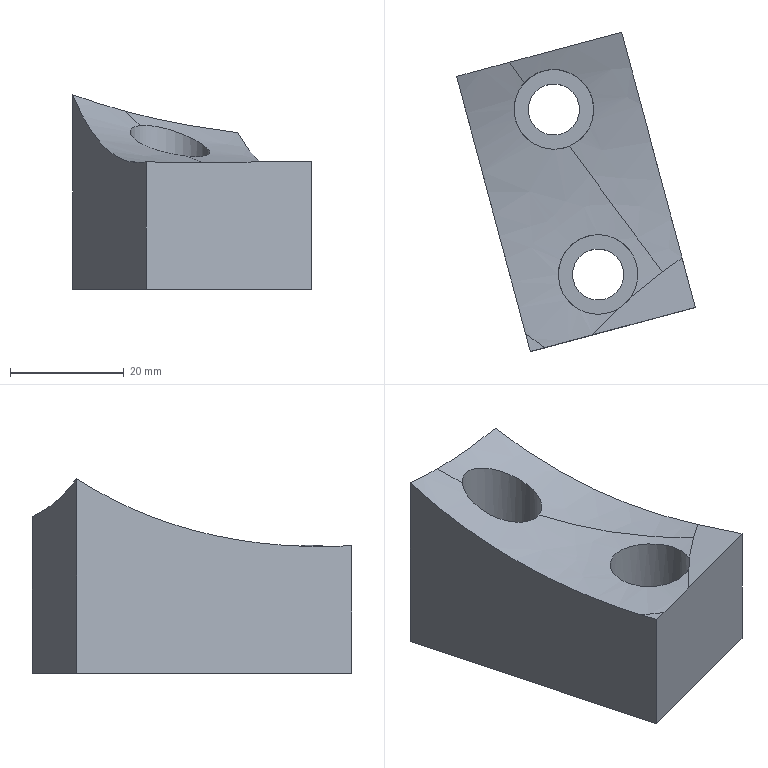Part | NX | features solid 2 | 1 solid | 15 faces | box 41.919 x 56.061 x 34.182 mm | volume 29881 mm3 | plane 7 | cylinder 4 | spline 4 | commonest cylinder face diameters 9 x2 14 x2
STEP:
#1=CARTESIAN_POINT('',(-500.421,532.504,-77.579));
#2=VERTEX_POINT('',#1);
#3=CARTESIAN_POINT('',(-497.915,533.175,-77.679));
#4=VERTEX_POINT('',#3);
#5=CARTESIAN_POINT('',(-500.421,532.504,-77.579));
#6=CARTESIAN_POINT('',(-499.586,532.727,-77.618));
#7=CARTESIAN_POINT('',(-498.751,532.951,-77.652));
#8=CARTESIAN_POINT('',(-497.915,533.175,-77.679));
#9=B_SPLINE_CURVE_WITH_KNOTS('',3,(#5,#6,#7,#8),.UNSPECIFIED.,.F.,.F.,(4,4),(0.,0.002596),.UNSPECIFIED.);
#10=EDGE_CURVE('',#2,#4,#9,.T.);
#11=ORIENTED_EDGE('',*,*,#10,.F.);
#12=CARTESIAN_POINT('',(-500.421,532.504,-100.));
#13=VERTEX_POINT('',#12);
#14=CARTESIAN_POINT('',(-500.421,532.504,-105.));
#15=DIRECTION('',(0.,0.,1.));
#16=VECTOR('',#15,1000.);
#17=LINE('',#14,#16);
#18=EDGE_CURVE('',#13,#2,#17,.T.);
#19=ORIENTED_EDGE('',*,*,#18,.F.);
#20=CARTESIAN_POINT('',(-471.443,540.268,-100.));
#21=VERTEX_POINT('',#20);
#22=CARTESIAN_POINT('',(-500.421,532.504,-100.));
#23=DIRECTION('',(0.9659,0.2588,0.));
#24=VECTOR('',#23,1000.);
#25=LINE('',#22,#24);
#26=EDGE_CURVE('',#13,#21,#25,.T.);
#27=ORIENTED_EDGE('',*,*,#26,.T.);
#28=CARTESIAN_POINT('',(-471.443,540.268,-77.491));
#29=VERTEX_POINT('',#28);
#30=CARTESIAN_POINT('',(-471.443,540.268,-105.));
#31=DIRECTION('',(0.,0.,1.));
#32=VECTOR('',#31,1000.);
#33=LINE('',#30,#32);
#34=EDGE_CURVE('',#21,#29,#33,.T.);
#35=ORIENTED_EDGE('',*,*,#34,.T.);
#36=CARTESIAN_POINT('',(-489.455,535.442,-77.745));
#37=VERTEX_POINT('',#36);
#38=CARTESIAN_POINT('',(-489.455,535.442,-77.745));
#39=CARTESIAN_POINT('',(-483.451,537.051,-77.658));
#40=CARTESIAN_POINT('',(-477.447,538.66,-77.574));
#41=CARTESIAN_POINT('',(-471.443,540.268,-77.491));
#42=B_SPLINE_CURVE_WITH_KNOTS('',3,(#38,#39,#40,#41),.UNSPECIFIED.,.F.,.F.,(4,4),(0.01135,0.03),.UNSPECIFIED.);
#43=EDGE_CURVE('',#37,#29,#42,.T.);
#44=ORIENTED_EDGE('',*,*,#43,.F.);
#45=CARTESIAN_POINT('',(-497.915,533.175,-77.679));
#46=CARTESIAN_POINT('',(-495.095,533.931,-77.77));
#47=CARTESIAN_POINT('',(-492.274,534.687,-77.786));
#48=CARTESIAN_POINT('',(-489.453,535.442,-77.745));
#49=B_SPLINE_CURVE_WITH_KNOTS('',3,(#45,#46,#47,#48),.UNSPECIFIED.,.F.,.F.,(4,4),(0.,0.008761),.UNSPECIFIED.);
#50=EDGE_CURVE('',#4,#37,#49,.T.);
#51=ORIENTED_EDGE('',*,*,#50,.F.);
#52=EDGE_LOOP('',(#11,#19,#27,#35,#44,#51));
#53=FACE_BOUND('',#52,.T.);
#54=CARTESIAN_POINT('',(-500.421,532.504,-105.));
#55=DIRECTION('',(0.2588,-0.9659,0.));
#56=DIRECTION('',(0.9659,0.2588,0.));
#57=AXIS2_PLACEMENT_3D('',#54,#55,#56);
#58=PLANE('',#57);
#59=ADVANCED_FACE('',(#53),#58,.T.);
#60=CARTESIAN_POINT('',(-473.762,548.924,-78.67));
#61=VERTEX_POINT('',#60);
#62=CARTESIAN_POINT('',(-484.384,588.565,-72.498));
#63=VERTEX_POINT('',#62);
#64=CARTESIAN_POINT('',(-473.762,548.921,-78.67));
#65=CARTESIAN_POINT('',(-475.574,555.683,-79.599));
#66=CARTESIAN_POINT('',(-478.278,565.777,-79.565));
#67=CARTESIAN_POINT('',(-481.86,579.146,-76.501));
#68=CARTESIAN_POINT('',(-483.556,585.475,-73.999));
#69=CARTESIAN_POINT('',(-484.384,588.565,-72.498));
#70=B_SPLINE_CURVE_WITH_KNOTS('',3,(#64,#65,#66,#67,#68,#69),.UNSPECIFIED.,.F.,.F.,(4,1,1,4),(0.,0.0209,0.03134,0.04179),.UNSPECIFIED.);
#71=EDGE_CURVE('',#61,#63,#70,.T.);
#72=ORIENTED_EDGE('',*,*,#71,.F.);
#73=CARTESIAN_POINT('',(-471.443,540.268,-77.491));
#74=CARTESIAN_POINT('',(-472.216,543.154,-77.881));
#75=CARTESIAN_POINT('',(-472.99,546.039,-78.274));
#76=CARTESIAN_POINT('',(-473.763,548.924,-78.67));
#77=B_SPLINE_CURVE_WITH_KNOTS('',3,(#73,#74,#75,#76),.UNSPECIFIED.,.F.,.F.,(4,4),(0.,0.009039),.UNSPECIFIED.);
#78=EDGE_CURVE('',#29,#61,#77,.T.);
#79=ORIENTED_EDGE('',*,*,#78,.F.);
#80=ORIENTED_EDGE('',*,*,#34,.F.);
#81=CARTESIAN_POINT('',(-484.384,588.565,-100.));
#82=VERTEX_POINT('',#81);
#83=CARTESIAN_POINT('',(-471.443,540.268,-100.));
#84=DIRECTION('',(-0.2588,0.9659,0.));
#85=VECTOR('',#84,1000.);
#86=LINE('',#83,#85);
#87=EDGE_CURVE('',#21,#82,#86,.T.);
#88=ORIENTED_EDGE('',*,*,#87,.T.);
#89=CARTESIAN_POINT('',(-484.384,588.565,-105.));
#90=DIRECTION('',(0.,0.,1.));
#91=VECTOR('',#90,1000.);
#92=LINE('',#89,#91);
#93=EDGE_CURVE('',#82,#63,#92,.T.);
#94=ORIENTED_EDGE('',*,*,#93,.T.);
#95=EDGE_LOOP('',(#72,#79,#80,#88,#94));
#96=FACE_BOUND('',#95,.T.);
#97=CARTESIAN_POINT('',(-471.443,540.268,-105.));
#98=DIRECTION('',(0.9659,0.2588,0.));
#99=DIRECTION('',(-0.2588,0.9659,0.));
#100=AXIS2_PLACEMENT_3D('',#97,#98,#99);
#101=PLANE('',#100);
#102=ADVANCED_FACE('',(#96),#101,.T.);
#103=CARTESIAN_POINT('',(-504.086,583.285,-68.736));
#104=VERTEX_POINT('',#103);
#105=CARTESIAN_POINT('',(-484.384,588.565,-72.498));
#106=CARTESIAN_POINT('',(-491.031,586.784,-71.689));
#107=CARTESIAN_POINT('',(-497.606,585.022,-70.481));
#108=CARTESIAN_POINT('',(-504.086,583.285,-68.736));
#109=B_SPLINE_CURVE_WITH_KNOTS('',3,(#105,#106,#107,#108),.UNSPECIFIED.,.F.,.F.,(4,4),(0.,0.02074),.UNSPECIFIED.);
#110=EDGE_CURVE('',#63,#104,#109,.T.);
#111=ORIENTED_EDGE('',*,*,#110,.F.);
#112=ORIENTED_EDGE('',*,*,#93,.F.);
#113=CARTESIAN_POINT('',(-513.362,580.8,-100.));
#114=VERTEX_POINT('',#113);
#115=CARTESIAN_POINT('',(-513.362,580.8,-100.));
#116=DIRECTION('',(-0.9659,-0.2588,0.));
#117=VECTOR('',#116,1000.);
#118=LINE('',#115,#117);
#119=EDGE_CURVE('',#114,#82,#118,.F.);
#120=ORIENTED_EDGE('',*,*,#119,.F.);
#121=CARTESIAN_POINT('',(-513.362,580.8,-65.818));
#122=VERTEX_POINT('',#121);
#123=CARTESIAN_POINT('',(-513.362,580.8,-105.));
#124=DIRECTION('',(0.,0.,1.));
#125=VECTOR('',#124,1000.);
#126=LINE('',#123,#125);
#127=EDGE_CURVE('',#114,#122,#126,.T.);
#128=ORIENTED_EDGE('',*,*,#127,.T.);
#129=CARTESIAN_POINT('',(-504.086,583.285,-68.736));
#130=CARTESIAN_POINT('',(-507.216,582.447,-67.893));
#131=CARTESIAN_POINT('',(-510.31,581.618,-66.926));
#132=CARTESIAN_POINT('',(-513.362,580.8,-65.818));
#133=B_SPLINE_CURVE_WITH_KNOTS('',3,(#129,#130,#131,#132),.UNSPECIFIED.,.F.,.F.,(4,4),(0.,0.01004),.UNSPECIFIED.);
#134=EDGE_CURVE('',#104,#122,#133,.T.);
#135=ORIENTED_EDGE('',*,*,#134,.F.);
#136=EDGE_LOOP('',(#111,#112,#120,#128,#135));
#137=FACE_BOUND('',#136,.T.);
#138=CARTESIAN_POINT('',(-513.362,580.8,-105.));
#139=DIRECTION('',(0.2588,-0.9659,0.));
#140=DIRECTION('',(0.9659,0.2588,0.));
#141=AXIS2_PLACEMENT_3D('',#138,#139,#140);
#142=PLANE('',#141);
#143=ADVANCED_FACE('',(#137),#142,.F.);
#144=CARTESIAN_POINT('',(-501.268,535.665,-77.703));
#145=VERTEX_POINT('',#144);
#146=CARTESIAN_POINT('',(-501.268,535.665,-77.703));
#147=CARTESIAN_POINT('',(-500.985,534.61,-77.677));
#148=CARTESIAN_POINT('',(-500.703,533.557,-77.636));
#149=CARTESIAN_POINT('',(-500.421,532.504,-77.579));
#150=B_SPLINE_CURVE_WITH_KNOTS('',3,(#146,#147,#148,#149),.UNSPECIFIED.,.F.,.F.,(4,4),(0.,0.003275),.UNSPECIFIED.);
#151=EDGE_CURVE('',#145,#2,#150,.T.);
#152=ORIENTED_EDGE('',*,*,#151,.F.);
#153=CARTESIAN_POINT('',(-513.362,580.8,-65.818));
#154=CARTESIAN_POINT('',(-511.553,574.049,-70.183));
#155=CARTESIAN_POINT('',(-508.654,563.228,-74.769));
#156=CARTESIAN_POINT('',(-504.446,547.527,-77.527));
#157=CARTESIAN_POINT('',(-502.331,539.632,-77.8));
#158=CARTESIAN_POINT('',(-501.268,535.665,-77.703));
#159=B_SPLINE_CURVE_WITH_KNOTS('',3,(#153,#154,#155,#156,#157,#158),.UNSPECIFIED.,.F.,.F.,(4,1,1,4),(0.,0.02423,0.03634,0.04846),.UNSPECIFIED.);
#160=EDGE_CURVE('',#122,#145,#159,.T.);
#161=ORIENTED_EDGE('',*,*,#160,.F.);
#162=ORIENTED_EDGE('',*,*,#127,.F.);
#163=CARTESIAN_POINT('',(-500.421,532.504,-100.));
#164=DIRECTION('',(0.2588,-0.9659,0.));
#165=VECTOR('',#164,1000.);
#166=LINE('',#163,#165);
#167=EDGE_CURVE('',#13,#114,#166,.F.);
#168=ORIENTED_EDGE('',*,*,#167,.F.);
#169=ORIENTED_EDGE('',*,*,#18,.T.);
#170=EDGE_LOOP('',(#152,#161,#162,#168,#169));
#171=FACE_BOUND('',#170,.T.);
#172=CARTESIAN_POINT('',(-500.421,532.504,-105.));
#173=DIRECTION('',(0.9659,0.2588,0.));
#174=DIRECTION('',(-0.2588,0.9659,0.));
#175=AXIS2_PLACEMENT_3D('',#172,#173,#174);
#176=PLANE('',#175);
#177=ADVANCED_FACE('',(#171),#176,.F.);
#178=CARTESIAN_POINT('',(-484.02,546.045,-100.));
#179=VERTEX_POINT('',#178);
#180=CARTESIAN_POINT('',(-488.52,546.045,-100.));
#181=DIRECTION('',(0.,0.,1.));
#182=DIRECTION('',(1.,0.,0.));
#183=AXIS2_PLACEMENT_3D('',#180,#181,#182);
#184=CIRCLE('',#183,4.5);
#185=EDGE_CURVE('',#179,#179,#184,.T.);
#186=ORIENTED_EDGE('',*,*,#185,.T.);
#187=EDGE_LOOP('',(#186));
#188=FACE_BOUND('',#187,.T.);
#189=CARTESIAN_POINT('',(-491.785,575.023,-100.));
#190=VERTEX_POINT('',#189);
#191=CARTESIAN_POINT('',(-496.285,575.023,-100.));
#192=DIRECTION('',(0.,0.,1.));
#193=DIRECTION('',(1.,0.,0.));
#194=AXIS2_PLACEMENT_3D('',#191,#192,#193);
#195=CIRCLE('',#194,4.5);
#196=EDGE_CURVE('',#190,#190,#195,.T.);
#197=ORIENTED_EDGE('',*,*,#196,.T.);
#198=EDGE_LOOP('',(#197));
#199=FACE_BOUND('',#198,.T.);
#200=ORIENTED_EDGE('',*,*,#119,.T.);
#201=ORIENTED_EDGE('',*,*,#87,.F.);
#202=ORIENTED_EDGE('',*,*,#26,.F.);
#203=ORIENTED_EDGE('',*,*,#167,.T.);
#204=EDGE_LOOP('',(#200,#201,#202,#203));
#205=FACE_BOUND('',#204,.T.);
#206=CARTESIAN_POINT('',(-500.421,532.504,-100.));
#207=DIRECTION('',(0.,0.,1.));
#208=DIRECTION('',(0.9659,0.2588,0.));
#209=AXIS2_PLACEMENT_3D('',#206,#207,#208);
#210=PLANE('',#209);
#211=ADVANCED_FACE('',(#188,#199,#205),#210,.F.);
#212=CARTESIAN_POINT('',(-500.785,575.023,-90.));
#213=VERTEX_POINT('',#212);
#214=CARTESIAN_POINT('',(-496.285,575.023,-90.));
#215=DIRECTION('',(0.,0.,-1.));
#216=DIRECTION('',(-1.,0.,0.));
#217=AXIS2_PLACEMENT_3D('',#214,#215,#216);
#218=CIRCLE('',#217,4.5);
#219=EDGE_CURVE('',#213,#213,#218,.T.);
#220=ORIENTED_EDGE('',*,*,#219,.F.);
#221=EDGE_LOOP('',(#220));
#222=FACE_BOUND('',#221,.T.);
#223=ORIENTED_EDGE('',*,*,#196,.F.);
#224=EDGE_LOOP('',(#223));
#225=FACE_BOUND('',#224,.T.);
#226=CARTESIAN_POINT('',(-496.285,575.023,-155.));
#227=DIRECTION('',(0.,0.,-1.));
#228=DIRECTION('',(-0.9659,-0.2588,0.));
#229=AXIS2_PLACEMENT_3D('',#226,#227,#228);
#230=CYLINDRICAL_SURFACE('',#229,4.5);
#231=ADVANCED_FACE('',(#222,#225),#230,.F.);
#232=ORIENTED_EDGE('',*,*,#219,.T.);
#233=EDGE_LOOP('',(#232));
#234=FACE_BOUND('',#233,.T.);
#235=CARTESIAN_POINT('',(-503.285,575.023,-90.));
#236=VERTEX_POINT('',#235);
#237=CARTESIAN_POINT('',(-496.285,575.023,-90.));
#238=DIRECTION('',(0.,0.,-1.));
#239=DIRECTION('',(-1.,0.,0.));
#240=AXIS2_PLACEMENT_3D('',#237,#238,#239);
#241=CIRCLE('',#240,7.);
#242=EDGE_CURVE('',#236,#236,#241,.T.);
#243=ORIENTED_EDGE('',*,*,#242,.F.);
#244=EDGE_LOOP('',(#243));
#245=FACE_BOUND('',#244,.T.);
#246=CARTESIAN_POINT('',(-496.285,575.023,-90.));
#247=DIRECTION('',(0.,0.,-1.));
#248=DIRECTION('',(-0.9659,-0.2588,0.));
#249=AXIS2_PLACEMENT_3D('',#246,#247,#248);
#250=PLANE('',#249);
#251=ADVANCED_FACE('',(#234,#245),#250,.F.);
#252=CARTESIAN_POINT('',(-501.518,579.672,-71.241));
#253=VERTEX_POINT('',#252);
#254=CARTESIAN_POINT('',(-493.533,568.587,-76.591));
#255=VERTEX_POINT('',#254);
#256=CARTESIAN_POINT('',(-501.518,579.672,-71.241));
#257=CARTESIAN_POINT('',(-502.619,578.433,-71.358));
#258=CARTESIAN_POINT('',(-503.814,575.269,-72.157));
#259=CARTESIAN_POINT('',(-502.402,570.664,-74.051));
#260=CARTESIAN_POINT('',(-498.459,567.796,-75.764));
#261=CARTESIAN_POINT('',(-495.053,567.937,-76.426));
#262=CARTESIAN_POINT('',(-493.533,568.587,-76.591));
#263=B_SPLINE_CURVE_WITH_KNOTS('',3,(#256,#257,#258,#259,#260,#261,#262),.UNSPECIFIED.,.F.,.F.,(4,1,1,1,4),(0.,0.004909,0.009818,0.01473,0.01964),.UNSPECIFIED.);
#264=EDGE_CURVE('',#253,#255,#263,.T.);
#265=ORIENTED_EDGE('',*,*,#264,.T.);
#266=CARTESIAN_POINT('',(-493.533,568.587,-76.591));
#267=CARTESIAN_POINT('',(-492.535,569.013,-76.698));
#268=CARTESIAN_POINT('',(-490.756,570.328,-76.767));
#269=CARTESIAN_POINT('',(-489.248,573.282,-76.412));
#270=CARTESIAN_POINT('',(-489.21,576.52,-75.612));
#271=CARTESIAN_POINT('',(-490.938,580.294,-74.127));
#272=CARTESIAN_POINT('',(-494.707,582.395,-72.345));
#273=CARTESIAN_POINT('',(-498.971,581.756,-71.261));
#274=CARTESIAN_POINT('',(-500.794,580.487,-71.165));
#275=CARTESIAN_POINT('',(-501.518,579.672,-71.241));
#276=B_SPLINE_CURVE_WITH_KNOTS('',3,(#266,#267,#268,#269,#270,#271,#272,#273,#274,#275),.UNSPECIFIED.,.F.,.F.,(4,1,1,1,1,1,1,4),(0.,0.003227,0.006454,0.009681,0.01291,0.01936,0.02259,0.02581),.UNSPECIFIED.);
#277=EDGE_CURVE('',#255,#253,#276,.T.);
#278=ORIENTED_EDGE('',*,*,#277,.T.);
#279=EDGE_LOOP('',(#265,#278));
#280=FACE_BOUND('',#279,.T.);
#281=ORIENTED_EDGE('',*,*,#242,.T.);
#282=EDGE_LOOP('',(#281));
#283=FACE_BOUND('',#282,.T.);
#284=CARTESIAN_POINT('',(-496.285,575.023,-5.));
#285=DIRECTION('',(0.,0.,-1.));
#286=DIRECTION('',(-0.9659,-0.2588,0.));
#287=AXIS2_PLACEMENT_3D('',#284,#285,#286);
#288=CYLINDRICAL_SURFACE('',#287,7.);
#289=ADVANCED_FACE('',(#280,#283),#288,.F.);
#290=CARTESIAN_POINT('',(-493.02,546.045,-90.));
#291=VERTEX_POINT('',#290);
#292=CARTESIAN_POINT('',(-488.52,546.045,-90.));
#293=DIRECTION('',(0.,0.,-1.));
#294=DIRECTION('',(-1.,0.,0.));
#295=AXIS2_PLACEMENT_3D('',#292,#293,#294);
#296=CIRCLE('',#295,4.5);
#297=EDGE_CURVE('',#291,#291,#296,.T.);
#298=ORIENTED_EDGE('',*,*,#297,.F.);
#299=EDGE_LOOP('',(#298));
#300=FACE_BOUND('',#299,.T.);
#301=ORIENTED_EDGE('',*,*,#185,.F.);
#302=EDGE_LOOP('',(#301));
#303=FACE_BOUND('',#302,.T.);
#304=CARTESIAN_POINT('',(-488.52,546.045,-155.));
#305=DIRECTION('',(0.,0.,-1.));
#306=DIRECTION('',(-0.9659,-0.2588,0.));
#307=AXIS2_PLACEMENT_3D('',#304,#305,#306);
#308=CYLINDRICAL_SURFACE('',#307,4.5);
#309=ADVANCED_FACE('',(#300,#303),#308,.F.);
#310=ORIENTED_EDGE('',*,*,#297,.T.);
#311=EDGE_LOOP('',(#310));
#312=FACE_BOUND('',#311,.T.);
#313=CARTESIAN_POINT('',(-495.52,546.045,-90.));
#314=VERTEX_POINT('',#313);
#315=CARTESIAN_POINT('',(-488.52,546.045,-90.));
#316=DIRECTION('',(0.,0.,-1.));
#317=DIRECTION('',(-1.,0.,0.));
#318=AXIS2_PLACEMENT_3D('',#315,#316,#317);
#319=CIRCLE('',#318,7.);
#320=EDGE_CURVE('',#314,#314,#319,.T.);
#321=ORIENTED_EDGE('',*,*,#320,.F.);
#322=EDGE_LOOP('',(#321));
#323=FACE_BOUND('',#322,.T.);
#324=CARTESIAN_POINT('',(-488.52,546.045,-90.));
#325=DIRECTION('',(0.,0.,-1.));
#326=DIRECTION('',(-0.9659,-0.2588,0.));
#327=AXIS2_PLACEMENT_3D('',#324,#325,#326);
#328=PLANE('',#327);
#329=ADVANCED_FACE('',(#312,#323),#328,.F.);
#330=CARTESIAN_POINT('',(-485.115,539.929,-78.089));
#331=VERTEX_POINT('',#330);
#332=CARTESIAN_POINT('',(-482.722,542.124,-78.246));
#333=VERTEX_POINT('',#332);
#334=CARTESIAN_POINT('',(-485.113,539.931,-78.089));
#335=CARTESIAN_POINT('',(-484.161,540.461,-78.109));
#336=CARTESIAN_POINT('',(-483.333,541.22,-78.164));
#337=CARTESIAN_POINT('',(-482.723,542.123,-78.246));
#338=B_SPLINE_CURVE_WITH_KNOTS('',3,(#334,#335,#336,#337),.UNSPECIFIED.,.F.,.F.,(4,4),(0.01271,0.01598),.UNSPECIFIED.);
#339=EDGE_CURVE('',#331,#333,#338,.T.);
#340=ORIENTED_EDGE('',*,*,#339,.T.);
#341=CARTESIAN_POINT('',(-482.721,542.125,-78.246));
#342=CARTESIAN_POINT('',(-481.764,543.541,-78.376));
#343=CARTESIAN_POINT('',(-480.949,547.027,-78.771));
#344=CARTESIAN_POINT('',(-483.511,551.824,-79.091));
#345=CARTESIAN_POINT('',(-488.62,553.687,-78.831));
#346=CARTESIAN_POINT('',(-493.664,551.698,-78.44));
#347=CARTESIAN_POINT('',(-496.124,546.847,-78.324));
#348=CARTESIAN_POINT('',(-494.732,541.584,-78.344));
#349=CARTESIAN_POINT('',(-490.184,538.588,-78.164));
#350=CARTESIAN_POINT('',(-486.614,539.095,-78.057));
#351=CARTESIAN_POINT('',(-485.117,539.928,-78.089));
#352=B_SPLINE_CURVE_WITH_KNOTS('',3,(#341,#342,#343,#344,#345,#346,#347,#348,#349,#350,#351),.UNSPECIFIED.,.F.,.F.,(4,1,1,1,1,1,1,1,4),(0.000003459,0.005072,0.01014,0.01521,0.02028,0.02535,0.03042,0.03549,0.04056),.UNSPECIFIED.);
#353=EDGE_CURVE('',#333,#331,#352,.T.);
#354=ORIENTED_EDGE('',*,*,#353,.T.);
#355=EDGE_LOOP('',(#340,#354));
#356=FACE_BOUND('',#355,.T.);
#357=ORIENTED_EDGE('',*,*,#320,.T.);
#358=EDGE_LOOP('',(#357));
#359=FACE_BOUND('',#358,.T.);
#360=CARTESIAN_POINT('',(-488.52,546.045,-5.));
#361=DIRECTION('',(0.,0.,-1.));
#362=DIRECTION('',(-0.9659,-0.2588,0.));
#363=AXIS2_PLACEMENT_3D('',#360,#361,#362);
#364=CYLINDRICAL_SURFACE('',#363,7.);
#365=ADVANCED_FACE('',(#356,#359),#364,.F.);
#366=CARTESIAN_POINT('',(-477.243,546.52,-78.534));
#367=VERTEX_POINT('',#366);
#368=CARTESIAN_POINT('',(-477.243,546.52,-78.534));
#369=CARTESIAN_POINT('',(-476.102,547.354,-78.584));
#370=CARTESIAN_POINT('',(-474.942,548.155,-78.629));
#371=CARTESIAN_POINT('',(-473.763,548.924,-78.67));
#372=B_SPLINE_CURVE_WITH_KNOTS('',3,(#368,#369,#370,#371),.UNSPECIFIED.,.F.,.F.,(4,4),(0.,0.09786),.UNSPECIFIED.);
#373=EDGE_CURVE('',#367,#61,#372,.T.);
#374=ORIENTED_EDGE('',*,*,#373,.T.);
#375=ORIENTED_EDGE('',*,*,#71,.T.);
#376=ORIENTED_EDGE('',*,*,#110,.T.);
#377=CARTESIAN_POINT('',(-501.518,579.672,-71.241));
#378=CARTESIAN_POINT('',(-502.393,580.899,-70.46));
#379=CARTESIAN_POINT('',(-503.25,582.105,-69.624));
#380=CARTESIAN_POINT('',(-504.086,583.285,-68.736));
#381=B_SPLINE_CURVE_WITH_KNOTS('',3,(#377,#378,#379,#380),.UNSPECIFIED.,.F.,.F.,(4,4),(0.6802,0.762),.UNSPECIFIED.);
#382=EDGE_CURVE('',#253,#104,#381,.T.);
#383=ORIENTED_EDGE('',*,*,#382,.F.);
#384=ORIENTED_EDGE('',*,*,#277,.F.);
#385=CARTESIAN_POINT('',(-477.243,546.52,-78.534));
#386=CARTESIAN_POINT('',(-482.731,553.843,-79.701));
#387=CARTESIAN_POINT('',(-488.303,561.391,-79.036));
#388=CARTESIAN_POINT('',(-493.533,568.587,-76.591));
#389=B_SPLINE_CURVE_WITH_KNOTS('',3,(#385,#386,#387,#388),.UNSPECIFIED.,.F.,.F.,(4,4),(0.,0.4443),.UNSPECIFIED.);
#390=EDGE_CURVE('',#367,#255,#389,.T.);
#391=ORIENTED_EDGE('',*,*,#390,.F.);
#392=EDGE_LOOP('',(#374,#375,#376,#383,#384,#391));
#393=FACE_BOUND('',#392,.T.);
#394=CARTESIAN_POINT('',(-466.153,552.97,-78.822));
#395=CARTESIAN_POINT('',(-466.602,553.844,-78.945));
#396=CARTESIAN_POINT('',(-467.502,555.593,-79.19));
#397=CARTESIAN_POINT('',(-469.307,559.11,-79.47));
#398=CARTESIAN_POINT('',(-471.565,563.522,-79.52));
#399=CARTESIAN_POINT('',(-474.261,568.806,-79.069));
#400=CARTESIAN_POINT('',(-476.923,574.04,-78.119));
#401=CARTESIAN_POINT('',(-479.531,579.188,-76.673));
#402=CARTESIAN_POINT('',(-482.067,584.211,-74.744));
#403=CARTESIAN_POINT('',(-484.104,588.262,-72.741));
#404=CARTESIAN_POINT('',(-485.683,591.41,-70.922));
#405=CARTESIAN_POINT('',(-486.447,592.939,-69.92));
#406=CARTESIAN_POINT('',(-486.83,593.703,-69.419));
#407=CARTESIAN_POINT('',(-467.104,552.477,-78.804));
#408=CARTESIAN_POINT('',(-467.566,553.346,-78.927));
#409=CARTESIAN_POINT('',(-468.49,555.083,-79.172));
#410=CARTESIAN_POINT('',(-470.344,558.578,-79.451));
#411=CARTESIAN_POINT('',(-472.665,562.962,-79.498));
#412=CARTESIAN_POINT('',(-475.434,568.212,-79.044));
#413=CARTESIAN_POINT('',(-478.167,573.414,-78.089));
#414=CARTESIAN_POINT('',(-480.845,578.529,-76.638));
#415=CARTESIAN_POINT('',(-483.448,583.522,-74.705));
#416=CARTESIAN_POINT('',(-485.537,587.548,-72.696));
#417=CARTESIAN_POINT('',(-487.156,590.676,-70.873));
#418=CARTESIAN_POINT('',(-487.94,592.196,-69.868));
#419=CARTESIAN_POINT('',(-488.332,592.955,-69.366));
#420=CARTESIAN_POINT('',(-469.005,551.491,-78.769));
#421=CARTESIAN_POINT('',(-469.492,552.348,-78.891));
#422=CARTESIAN_POINT('',(-470.465,554.063,-79.135));
#423=CARTESIAN_POINT('',(-472.42,557.513,-79.411));
#424=CARTESIAN_POINT('',(-474.864,561.841,-79.455));
#425=CARTESIAN_POINT('',(-477.779,567.025,-78.993));
#426=CARTESIAN_POINT('',(-480.655,572.161,-78.031));
#427=CARTESIAN_POINT('',(-483.472,577.213,-76.57));
#428=CARTESIAN_POINT('',(-486.208,582.144,-74.625));
#429=CARTESIAN_POINT('',(-488.403,586.119,-72.606));
#430=CARTESIAN_POINT('',(-490.104,589.209,-70.774));
#431=CARTESIAN_POINT('',(-490.926,590.71,-69.766));
#432=CARTESIAN_POINT('',(-491.337,591.46,-69.261));
#433=CARTESIAN_POINT('',(-471.766,549.87,-78.694));
#434=CARTESIAN_POINT('',(-472.289,550.708,-78.815));
#435=CARTESIAN_POINT('',(-473.337,552.384,-79.058));
#436=CARTESIAN_POINT('',(-475.439,555.759,-79.329));
#437=CARTESIAN_POINT('',(-478.066,559.992,-79.364));
#438=CARTESIAN_POINT('',(-481.198,565.064,-78.891));
#439=CARTESIAN_POINT('',(-484.286,570.091,-77.913));
#440=CARTESIAN_POINT('',(-487.307,575.035,-76.436));
#441=CARTESIAN_POINT('',(-490.241,579.862,-74.473));
#442=CARTESIAN_POINT('',(-492.593,583.754,-72.437));
#443=CARTESIAN_POINT('',(-494.412,586.779,-70.59));
#444=CARTESIAN_POINT('',(-495.292,588.248,-69.574));
#445=CARTESIAN_POINT('',(-495.732,588.983,-69.065));
#446=CARTESIAN_POINT('',(-474.465,548.154,-78.606));
#447=CARTESIAN_POINT('',(-475.026,548.972,-78.726));
#448=CARTESIAN_POINT('',(-476.146,550.607,-78.966));
#449=CARTESIAN_POINT('',(-478.393,553.9,-79.231));
#450=CARTESIAN_POINT('',(-481.202,558.032,-79.257));
#451=CARTESIAN_POINT('',(-484.548,562.985,-78.77));
#452=CARTESIAN_POINT('',(-487.845,567.893,-77.777));
#453=CARTESIAN_POINT('',(-491.069,572.722,-76.282));
#454=CARTESIAN_POINT('',(-494.198,577.437,-74.298));
#455=CARTESIAN_POINT('',(-496.703,581.24,-72.243));
#456=CARTESIAN_POINT('',(-498.641,584.196,-70.381));
#457=CARTESIAN_POINT('',(-499.577,585.631,-69.357));
#458=CARTESIAN_POINT('',(-500.046,586.349,-68.844));
#459=CARTESIAN_POINT('',(-476.204,546.914,-78.533));
#460=CARTESIAN_POINT('',(-476.788,547.717,-78.652));
#461=CARTESIAN_POINT('',(-477.956,549.323,-78.89));
#462=CARTESIAN_POINT('',(-480.298,552.556,-79.15));
#463=CARTESIAN_POINT('',(-483.224,556.614,-79.169));
#464=CARTESIAN_POINT('',(-486.71,561.479,-78.672));
#465=CARTESIAN_POINT('',(-490.143,566.301,-77.667));
#466=CARTESIAN_POINT('',(-493.499,571.046,-76.158));
#467=CARTESIAN_POINT('',(-496.754,575.679,-74.159));
#468=CARTESIAN_POINT('',(-499.359,579.417,-72.091));
#469=CARTESIAN_POINT('',(-501.373,582.322,-70.218));
#470=CARTESIAN_POINT('',(-502.346,583.733,-69.187));
#471=CARTESIAN_POINT('',(-502.833,584.439,-68.672));
#472=CARTESIAN_POINT('',(-477.074,546.294,-78.497));
#473=CARTESIAN_POINT('',(-477.669,547.09,-78.615));
#474=CARTESIAN_POINT('',(-478.861,548.681,-78.852));
#475=CARTESIAN_POINT('',(-481.25,551.884,-79.11));
#476=CARTESIAN_POINT('',(-484.236,555.905,-79.126));
#477=CARTESIAN_POINT('',(-487.791,560.726,-78.623));
#478=CARTESIAN_POINT('',(-491.292,565.505,-77.612));
#479=CARTESIAN_POINT('',(-494.714,570.208,-76.096));
#480=CARTESIAN_POINT('',(-498.031,574.8,-74.09));
#481=CARTESIAN_POINT('',(-500.687,578.505,-72.015));
#482=CARTESIAN_POINT('',(-502.739,581.385,-70.136));
#483=CARTESIAN_POINT('',(-503.731,582.784,-69.103));
#484=CARTESIAN_POINT('',(-504.226,583.483,-68.586));
#485=B_SPLINE_SURFACE_WITH_KNOTS('',3,3,((#394,#395,#396,#397,#398,#399,#400,#401,#402,#403,#404,#405,#406),(#407,#408,#409,#410,#411,#412,#413,#414,#415,#416,#417,#418,#419),(#420,#421,#422,#423,#424,#425,#426,#427,#428,#429,#430,#431,#432),(#433,#434,#435,#436,#437,#438,#439,#440,#441,#442,#443,#444,#445),(#446,#447,#448,#449,#450,#451,#452,#453,#454,#455,#456,#457,#458),(#459,#460,#461,#462,#463,#464,#465,#466,#467,#468,#469,#470,#471),(#472,#473,#474,#475,#476,#477,#478,#479,#480,#481,#482,#483,#484)),.UNSPECIFIED.,.F.,.F.,.F.,(4,1,1,1,4),(4,1,1,1,1,1,1,1,1,1,4),(0.04343,0.04666,0.04989,0.05313,0.05636),(-0.004572,0.04362,0.09182,0.1882,0.2846,0.381,0.4774,0.5738,0.6702,0.7184,0.7666),.UNSPECIFIED.);
#486=ADVANCED_FACE('',(#393),#485,.F.);
#487=CARTESIAN_POINT('',(-497.071,538.492,-7.886));
#488=DIRECTION('',(0.5951,0.8008,-0.0682));
#489=DIRECTION('',(-0.8026,0.5965,0.));
#490=AXIS2_PLACEMENT_3D('',#487,#488,#489);
#491=CIRCLE('',#490,70.);
#492=EDGE_CURVE('',#4,#145,#491,.T.);
#493=ORIENTED_EDGE('',*,*,#492,.F.);
#494=ORIENTED_EDGE('',*,*,#50,.T.);
#495=CARTESIAN_POINT('',(-489.454,535.443,-77.745));
#496=CARTESIAN_POINT('',(-488.06,537.002,-77.869));
#497=CARTESIAN_POINT('',(-486.614,538.497,-77.984));
#498=CARTESIAN_POINT('',(-485.117,539.928,-78.089));
#499=B_SPLINE_CURVE_WITH_KNOTS('',3,(#495,#496,#497,#498),.UNSPECIFIED.,.F.,.F.,(4,4),(0.2896,0.5569),.UNSPECIFIED.);
#500=EDGE_CURVE('',#37,#331,#499,.T.);
#501=ORIENTED_EDGE('',*,*,#500,.T.);
#502=ORIENTED_EDGE('',*,*,#353,.F.);
#503=CARTESIAN_POINT('',(-482.722,542.124,-78.246));
#504=CARTESIAN_POINT('',(-480.962,543.672,-78.354));
#505=CARTESIAN_POINT('',(-479.136,545.137,-78.45));
#506=CARTESIAN_POINT('',(-477.243,546.52,-78.534));
#507=B_SPLINE_CURVE_WITH_KNOTS('',3,(#503,#504,#505,#506),.UNSPECIFIED.,.F.,.F.,(4,4),(0.6968,1.),.UNSPECIFIED.);
#508=EDGE_CURVE('',#333,#367,#507,.T.);
#509=ORIENTED_EDGE('',*,*,#508,.T.);
#510=ORIENTED_EDGE('',*,*,#390,.T.);
#511=ORIENTED_EDGE('',*,*,#264,.F.);
#512=ORIENTED_EDGE('',*,*,#382,.T.);
#513=ORIENTED_EDGE('',*,*,#134,.T.);
#514=ORIENTED_EDGE('',*,*,#160,.T.);
#515=EDGE_LOOP('',(#493,#494,#501,#502,#509,#510,#511,#512,#513,#514));
#516=FACE_BOUND('',#515,.T.);
#517=CARTESIAN_POINT('',(-477.243,546.52,-78.534));
#518=CARTESIAN_POINT('',(-493.502,568.214,-81.991));
#519=CARTESIAN_POINT('',(-506.319,586.45,-66.176));
#520=CARTESIAN_POINT('',(-483.643,541.844,-78.252));
#521=CARTESIAN_POINT('',(-502.302,562.01,-81.608));
#522=CARTESIAN_POINT('',(-516.829,579.067,-65.47));
#523=CARTESIAN_POINT('',(-489.121,536.35,-77.835));
#524=CARTESIAN_POINT('',(-509.86,554.676,-81.037));
#525=CARTESIAN_POINT('',(-525.849,570.327,-64.526));
#526=CARTESIAN_POINT('',(-493.803,530.151,-77.31));
#527=CARTESIAN_POINT('',(-516.218,546.55,-80.336));
#528=CARTESIAN_POINT('',(-533.372,560.735,-63.451));
#529=(BOUNDED_SURFACE()B_SPLINE_SURFACE(3,2,((#517,#518,#519),(#520,#521,#522),(#523,#524,#525),(#526,#527,#528)),.UNSPECIFIED.,.F.,.F.,.F.)B_SPLINE_SURFACE_WITH_KNOTS((4,4),(3,3),(0.02442,0.04808),(0.,0.8335),.PIECEWISE_BEZIER_KNOTS.)GEOMETRIC_REPRESENTATION_ITEM()RATIONAL_B_SPLINE_SURFACE(((1.,0.9188,0.973),(1.,0.9178,0.9726),(1.,0.9167,0.9722),(1.,0.9156,0.9719)))REPRESENTATION_ITEM('')SURFACE());
#530=ADVANCED_FACE('',(#516),#529,.F.);
#531=ORIENTED_EDGE('',*,*,#500,.F.);
#532=ORIENTED_EDGE('',*,*,#43,.T.);
#533=ORIENTED_EDGE('',*,*,#78,.T.);
#534=ORIENTED_EDGE('',*,*,#373,.F.);
#535=ORIENTED_EDGE('',*,*,#508,.F.);
#536=ORIENTED_EDGE('',*,*,#339,.F.);
#537=EDGE_LOOP('',(#531,#532,#533,#534,#535,#536));
#538=FACE_BOUND('',#537,.T.);
#539=CARTESIAN_POINT('',(-489.563,535.361,-77.74));
#540=CARTESIAN_POINT('',(-483.487,535.361,-77.455));
#541=CARTESIAN_POINT('',(-477.411,535.361,-77.17));
#542=CARTESIAN_POINT('',(-471.335,535.361,-76.887));
#543=CARTESIAN_POINT('',(-489.563,539.909,-78.293));
#544=CARTESIAN_POINT('',(-483.487,539.909,-78.007));
#545=CARTESIAN_POINT('',(-477.411,539.909,-77.722));
#546=CARTESIAN_POINT('',(-471.335,539.909,-77.439));
#547=CARTESIAN_POINT('',(-489.563,544.457,-78.853));
#548=CARTESIAN_POINT('',(-483.487,544.457,-78.567));
#549=CARTESIAN_POINT('',(-477.411,544.457,-78.282));
#550=CARTESIAN_POINT('',(-471.335,544.457,-77.999));
#551=CARTESIAN_POINT('',(-489.563,549.005,-79.422));
#552=CARTESIAN_POINT('',(-483.487,549.005,-79.136));
#553=CARTESIAN_POINT('',(-477.411,549.005,-78.851));
#554=CARTESIAN_POINT('',(-471.335,549.005,-78.567));
#555=B_SPLINE_SURFACE_WITH_KNOTS('',3,3,((#539,#540,#541,#542),(#543,#544,#545,#546),(#547,#548,#549,#550),(#551,#552,#553,#554)),.UNSPECIFIED.,.F.,.F.,.F.,(4,4),(4,4),(0.7022,0.7085),(0.3948,0.4021),.PIECEWISE_BEZIER_KNOTS.);
#556=ADVANCED_FACE('',(#538),#555,.F.);
#557=ORIENTED_EDGE('',*,*,#151,.T.);
#558=ORIENTED_EDGE('',*,*,#10,.T.);
#559=ORIENTED_EDGE('',*,*,#492,.T.);
#560=EDGE_LOOP('',(#557,#558,#559));
#561=FACE_BOUND('',#560,.T.);
#562=CARTESIAN_POINT('',(-497.895,533.16,-77.678));
#563=CARTESIAN_POINT('',(-499.594,534.416,-77.754));
#564=CARTESIAN_POINT('',(-501.288,535.68,-77.702));
#565=CARTESIAN_POINT('',(-498.306,532.617,-77.631));
#566=CARTESIAN_POINT('',(-500.006,533.874,-77.707));
#567=CARTESIAN_POINT('',(-501.7,535.137,-77.656));
#568=CARTESIAN_POINT('',(-498.718,532.074,-77.585));
#569=CARTESIAN_POINT('',(-500.417,533.331,-77.661));
#570=CARTESIAN_POINT('',(-502.112,534.595,-77.609));
#571=CARTESIAN_POINT('',(-499.129,531.532,-77.539));
#572=CARTESIAN_POINT('',(-500.829,532.789,-77.615));
#573=CARTESIAN_POINT('',(-502.524,534.053,-77.562));
#574=(BOUNDED_SURFACE()B_SPLINE_SURFACE(3,2,((#562,#563,#564),(#565,#566,#567),(#568,#569,#570),(#571,#572,#573)),.UNSPECIFIED.,.F.,.F.,.F.)B_SPLINE_SURFACE_WITH_KNOTS((4,4),(3,3),(0.0554,0.05748),(0.08233,0.1498),.PIECEWISE_BEZIER_KNOTS.)GEOMETRIC_REPRESENTATION_ITEM()RATIONAL_B_SPLINE_SURFACE(((0.9847,0.979,0.9742),(0.9847,0.979,0.9742),(0.9847,0.979,0.9742),(0.9847,0.979,0.9742)))REPRESENTATION_ITEM('')SURFACE());
#575=ADVANCED_FACE('',(#561),#574,.F.);
#576=CLOSED_SHELL('',(#59,#102,#143,#177,#211,#231,#251,#289,#309,#329,#365,#486,#530,#556,#575));
#577=MANIFOLD_SOLID_BREP('',#576);
#578=(LENGTH_UNIT()NAMED_UNIT(*)SI_UNIT(.MILLI.,.METRE.));
#579=UNCERTAINTY_MEASURE_WITH_UNIT(LENGTH_MEASURE(0.1016),#578,'','');
#580=(NAMED_UNIT(*)PLANE_ANGLE_UNIT()SI_UNIT($,.RADIAN.));
#581=(NAMED_UNIT(*)SI_UNIT($,.STERADIAN.)SOLID_ANGLE_UNIT());
#582=(GEOMETRIC_REPRESENTATION_CONTEXT(3)GLOBAL_UNCERTAINTY_ASSIGNED_CONTEXT((#579))GLOBAL_UNIT_ASSIGNED_CONTEXT((#578,#580,#581))REPRESENTATION_CONTEXT('',''));
#583=ADVANCED_BREP_SHAPE_REPRESENTATION('',(#577),#582);